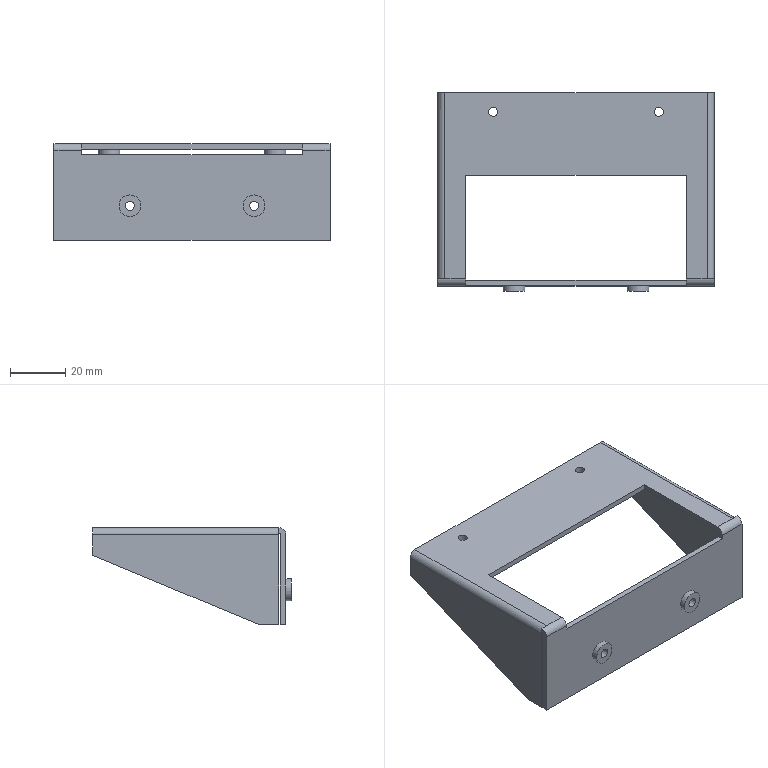Part | STEP file | 1 solid | 44 faces | box 100 x 72 x 35 mm | volume 19846 mm3 | plane 28 | cylinder 16 | commonest cylinder face diameters 1 x4 3.3 x4 5 x4 7.9 x4